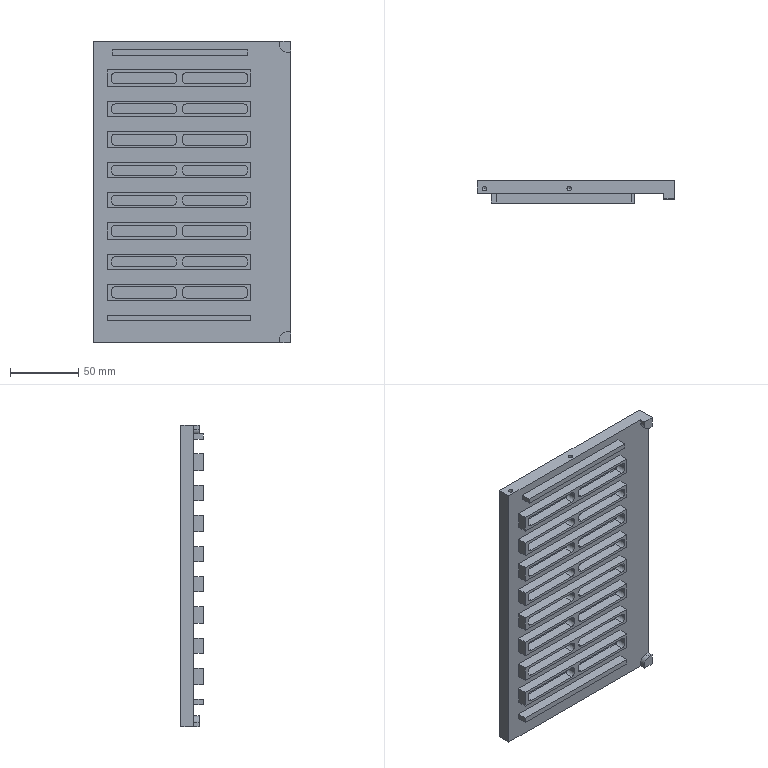NC program | NX | posted with a generic post | part box 144.5 x 16.5 x 221 mm
Lines 28 to 872 of 2050:
(PLANAR_MILL_9_COPY , TOOL : D2-6-D4-50-3T-FINISH)
N48 T13 M6
N50 G54
N52 G17 G0 G90 X66.787 Y-5.37 S4500 M3
N54 G43 Z20. H13
N56 Z1.
N58 G94 G1 X66.766 Y-5.373 Z0.998 F600.
N60 X66.624 Y-5.434 Z0.985
N62 X66.499 Y-5.527 Z0.971
N64 X66.401 Y-5.647 Z0.957
N66 X66.333 Y-5.786 Z0.944
N68 X66.3 Y-5.937 Z0.93
N70 Y-6.063 Z0.919
N72 X66.333 Y-6.214 Z0.906
N74 X66.401 Y-6.353 Z0.892
N76 X66.499 Y-6.473 Z0.879
N78 X66.624 Y-6.566 Z0.865
N80 X66.766 Y-6.627 Z0.852
N82 X66.919 Y-6.652 Z0.838
N84 X67.073 Y-6.641 Z0.825
N86 X67.221 Y-6.594 Z0.811
N88 X67.329 Y-6.532 Z0.8
N90 X67.433 Y-6.439 Z0.788
N92 X67.516 Y-6.327 Z0.776
N94 X67.572 Y-6.199 Z0.763
N96 X67.6 Y-6.063 Z0.751
N98 Y-5.937 Z0.74
N100 X67.572 Y-5.801 Z0.728
N102 X67.516 Y-5.674 Z0.716
N104 X67.433 Y-5.561 Z0.704
N106 X67.329 Y-5.468 Z0.692
N108 X67.221 Y-5.406 Z0.681
N110 X67.073 Y-5.359 Z0.667
N112 X66.919 Y-5.348 Z0.654
N114 X66.766 Y-5.373 Z0.64
N116 X66.624 Y-5.434 Z0.626
N118 X66.499 Y-5.527 Z0.613
N120 X66.401 Y-5.647 Z0.599
N122 X66.333 Y-5.786 Z0.586
N124 X66.3 Y-5.937 Z0.572
N126 Y-6.063 Z0.561
N128 X66.333 Y-6.214 Z0.548
N130 X66.401 Y-6.353 Z0.534
N132 X66.499 Y-6.473 Z0.521
N134 X66.624 Y-6.566 Z0.507
N136 X66.766 Y-6.627 Z0.493
N138 X66.919 Y-6.652 Z0.48
N140 X67.073 Y-6.641 Z0.466
N142 X67.221 Y-6.594 Z0.453
N144 X67.329 Y-6.532 Z0.442
N146 X67.433 Y-6.439 Z0.43
N148 X67.516 Y-6.327 Z0.417
N150 X67.572 Y-6.199 Z0.405
N152 X67.6 Y-6.063 Z0.393
N154 Y-5.937 Z0.382
N156 X67.572 Y-5.801 Z0.37
N158 X67.516 Y-5.674 Z0.358
N160 X67.433 Y-5.561 Z0.346
N162 X67.329 Y-5.468 Z0.333
N164 X67.221 Y-5.406 Z0.322
N166 X67.073 Y-5.359 Z0.309
N168 X66.919 Y-5.348 Z0.295
N170 X66.766 Y-5.373 Z0.282
N172 X66.624 Y-5.434 Z0.268
N174 X66.499 Y-5.527 Z0.255
N176 X66.401 Y-5.647 Z0.241
N178 X66.333 Y-5.786 Z0.228
N180 X66.3 Y-5.937 Z0.214
N182 Y-6.063 Z0.203
N184 X66.333 Y-6.214 Z0.189
N186 X66.401 Y-6.353 Z0.176
N188 X66.499 Y-6.473 Z0.162
N190 X66.624 Y-6.566 Z0.149
N192 X66.766 Y-6.627 Z0.135
N194 X66.919 Y-6.652 Z0.122
N196 X67.073 Y-6.641 Z0.108
N198 X67.221 Y-6.594 Z0.095
N200 X67.329 Y-6.532 Z0.084
N202 X67.433 Y-6.439 Z0.071
N204 X67.516 Y-6.327 Z0.059
N206 X67.572 Y-6.199 Z0.047
N208 X67.6 Y-6.063 Z0.035
N210 Y-5.937 Z0.024
N212 X67.572 Y-5.801 Z0.012
N214 X67.516 Y-5.674 Z0.
N216 X67.433 Y-5.561 Z-0.013
N218 X67.329 Y-5.468 Z-0.025
N220 X67.221 Y-5.406 Z-0.036
N222 X67.073 Y-5.359 Z-0.049
N224 X66.919 Y-5.348 Z-0.063
N226 X66.766 Y-5.373 Z-0.076
N228 X66.624 Y-5.434 Z-0.09
N230 X66.499 Y-5.527 Z-0.104
N232 X66.401 Y-5.647 Z-0.117
N234 X66.333 Y-5.786 Z-0.131
N236 X66.3 Y-5.937 Z-0.144
N238 Y-6.063 Z-0.155
N240 X66.333 Y-6.214 Z-0.169
N242 X66.401 Y-6.353 Z-0.182
N244 X66.499 Y-6.473 Z-0.196
N246 X66.624 Y-6.566 Z-0.209
N248 X66.766 Y-6.627 Z-0.223
N250 X66.919 Y-6.652 Z-0.236
N252 X67.073 Y-6.641 Z-0.25
N254 X67.221 Y-6.594 Z-0.264
N256 X67.329 Y-6.532 Z-0.275
N258 X67.433 Y-6.439 Z-0.287
N260 X67.516 Y-6.327 Z-0.299
N262 X67.572 Y-6.199 Z-0.311
N264 X67.6 Y-6.063 Z-0.323
N266 Y-5.937 Z-0.334
N268 X67.572 Y-5.801 Z-0.346
N270 X67.516 Y-5.674 Z-0.359
N272 X67.433 Y-5.561 Z-0.371
N274 X67.329 Y-5.468 Z-0.383
N276 X67.221 Y-5.406 Z-0.394
N278 X67.073 Y-5.359 Z-0.408
N280 X66.919 Y-5.348 Z-0.421
N282 X66.766 Y-5.373 Z-0.435
N284 X66.624 Y-5.434 Z-0.448
N286 X66.499 Y-5.527 Z-0.462
N288 X66.401 Y-5.647 Z-0.475
N290 X66.333 Y-5.786 Z-0.489
N292 X66.3 Y-5.937 Z-0.502
N294 Y-6.063 Z-0.513
N296 X66.333 Y-6.214 Z-0.527
N298 X66.401 Y-6.353 Z-0.54
N300 X66.499 Y-6.473 Z-0.554
N302 X66.624 Y-6.566 Z-0.568
N304 X66.766 Y-6.627 Z-0.581
N306 X66.919 Y-6.652 Z-0.595
N308 X67.073 Y-6.641 Z-0.608
N310 X67.221 Y-6.594 Z-0.622
N312 X67.329 Y-6.532 Z-0.633
N314 X67.433 Y-6.439 Z-0.645
N316 X67.516 Y-6.327 Z-0.657
N318 X67.572 Y-6.199 Z-0.669
N320 X67.6 Y-6.063 Z-0.681
N322 Y-5.937 Z-0.692
N324 X67.572 Y-5.801 Z-0.705
N326 X67.516 Y-5.674 Z-0.717
N328 X67.433 Y-5.561 Z-0.729
N330 X67.329 Y-5.468 Z-0.741
N332 X67.221 Y-5.406 Z-0.752
N334 X67.073 Y-5.359 Z-0.766
N336 X66.919 Y-5.348 Z-0.779
N338 X66.766 Y-5.373 Z-0.793
N340 X66.624 Y-5.434 Z-0.806
N342 X66.499 Y-5.527 Z-0.82
N344 X66.401 Y-5.647 Z-0.833
N346 X66.333 Y-5.786 Z-0.847
N348 X66.3 Y-5.937 Z-0.861
N350 Y-6.063 Z-0.872
N352 X66.333 Y-6.214 Z-0.885
N354 X66.401 Y-6.353 Z-0.899
N356 X66.499 Y-6.473 Z-0.912
N358 X66.624 Y-6.566 Z-0.926
N360 X66.766 Y-6.627 Z-0.939
N362 X66.919 Y-6.652 Z-0.953
N364 X67.073 Y-6.641 Z-0.966
N366 X67.221 Y-6.594 Z-0.98
N368 X67.329 Y-6.532 Z-0.991
N370 X67.433 Y-6.439 Z-1.003
N372 X67.516 Y-6.327 Z-1.015
N374 X67.572 Y-6.199 Z-1.027
N376 X67.6 Y-6.063 Z-1.04
N378 Y-5.937 Z-1.051
N380 X67.572 Y-5.801 Z-1.063
N382 X67.516 Y-5.674 Z-1.075
N384 X67.433 Y-5.561 Z-1.087
N386 X67.329 Y-5.468 Z-1.099
N388 X67.221 Y-5.406 Z-1.11
N390 X67.073 Y-5.359 Z-1.124
N392 X66.919 Y-5.348 Z-1.137
N394 X66.766 Y-5.373 Z-1.151
N396 X66.624 Y-5.434 Z-1.165
N398 X66.499 Y-5.527 Z-1.178
N400 X66.401 Y-5.647 Z-1.192
N402 X66.333 Y-5.786 Z-1.205
N404 X66.3 Y-5.937 Z-1.219
N406 Y-6.063 Z-1.23
N408 X66.333 Y-6.214 Z-1.243
N410 X66.401 Y-6.353 Z-1.257
N412 X66.499 Y-6.473 Z-1.27
N414 X66.624 Y-6.566 Z-1.284
N416 X66.766 Y-6.627 Z-1.297
N418 X66.919 Y-6.652 Z-1.311
N420 X67.073 Y-6.641 Z-1.325
N422 X67.221 Y-6.594 Z-1.338
N424 X67.329 Y-6.532 Z-1.349
N426 X67.433 Y-6.439 Z-1.361
N428 X67.516 Y-6.327 Z-1.373
N430 X67.572 Y-6.199 Z-1.386
N432 X67.6 Y-6.063 Z-1.398
N434 Y-5.937 Z-1.409
N436 X67.572 Y-5.801 Z-1.421
N438 X67.516 Y-5.674 Z-1.433
N440 X67.433 Y-5.561 Z-1.445
N442 X67.329 Y-5.468 Z-1.458
N444 X67.221 Y-5.406 Z-1.469
N446 X67.073 Y-5.359 Z-1.482
N448 X66.919 Y-5.348 Z-1.496
N450 X66.766 Y-5.373 Z-1.509
N452 X66.624 Y-5.434 Z-1.523
N454 X66.499 Y-5.527 Z-1.536
N456 X66.401 Y-5.647 Z-1.55
N458 X66.333 Y-5.786 Z-1.563
N460 X66.3 Y-5.937 Z-1.577
N462 Y-6.063 Z-1.588
N464 X66.333 Y-6.214 Z-1.601
N466 X66.401 Y-6.353 Z-1.615
N468 X66.499 Y-6.473 Z-1.629
N470 X66.624 Y-6.566 Z-1.642
N472 X66.766 Y-6.627 Z-1.656
N474 X66.919 Y-6.652 Z-1.669
N476 X67.073 Y-6.641 Z-1.683
N478 X67.221 Y-6.594 Z-1.696
N480 X67.329 Y-6.532 Z-1.707
N482 X67.433 Y-6.439 Z-1.719
N484 X67.516 Y-6.327 Z-1.732
N486 X67.572 Y-6.199 Z-1.744
N488 X67.6 Y-6.063 Z-1.756
N490 Y-5.937 Z-1.767
N492 X67.572 Y-5.801 Z-1.779
N494 X67.516 Y-5.674 Z-1.791
N496 X67.433 Y-5.561 Z-1.804
N498 X67.329 Y-5.468 Z-1.816
N500 X67.221 Y-5.406 Z-1.827
N502 X67.073 Y-5.359 Z-1.84
N504 X66.919 Y-5.348 Z-1.854
N506 X66.766 Y-5.373 Z-1.867
N508 X66.624 Y-5.434 Z-1.881
N510 X66.499 Y-5.527 Z-1.895
N512 X66.401 Y-5.647 Z-1.908
N514 X66.333 Y-5.786 Z-1.922
N516 X66.3 Y-5.937 Z-1.935
N518 Y-6.063 Z-1.946
N520 X66.333 Y-6.214 Z-1.96
N522 X66.401 Y-6.353 Z-1.973
N524 X66.499 Y-6.473 Z-1.987
N526 X66.624 Y-6.566 Z-2.
N528 X66.766 Y-6.627 Z-2.014
N530 X66.919 Y-6.652 Z-2.027
N532 X67.073 Y-6.641 Z-2.041
N534 X67.221 Y-6.594 Z-2.055
N536 X67.329 Y-6.532 Z-2.065
N538 X67.433 Y-6.439 Z-2.078
N540 X67.516 Y-6.327 Z-2.09
N542 X67.572 Y-6.199 Z-2.102
N544 X67.6 Y-6.063 Z-2.114
N546 Y-5.937 Z-2.125
N548 X67.572 Y-5.801 Z-2.137
N550 X67.516 Y-5.674 Z-2.15
N552 X67.433 Y-5.561 Z-2.162
N554 X67.329 Y-5.468 Z-2.174
N556 X67.221 Y-5.406 Z-2.185
N558 X67.073 Y-5.359 Z-2.198
N560 X66.919 Y-5.348 Z-2.212
N562 X66.766 Y-5.373 Z-2.226
N564 X66.624 Y-5.434 Z-2.239
N566 X66.499 Y-5.527 Z-2.253
N568 X66.401 Y-5.647 Z-2.266
N570 X66.333 Y-5.786 Z-2.28
N572 X66.3 Y-5.937 Z-2.293
N574 Y-6.063 Z-2.304
N576 X66.333 Y-6.214 Z-2.318
N578 X66.401 Y-6.353 Z-2.331
N580 X66.499 Y-6.473 Z-2.345
N582 X66.624 Y-6.566 Z-2.359
N584 X66.766 Y-6.627 Z-2.372
N586 X66.919 Y-6.652 Z-2.386
N588 X67.073 Y-6.641 Z-2.399
N590 X67.221 Y-6.594 Z-2.413
N592 X67.329 Y-6.532 Z-2.424
N594 X67.433 Y-6.439 Z-2.436
N596 X67.516 Y-6.327 Z-2.448
N598 X67.572 Y-6.199 Z-2.46
N600 X67.6 Y-6.063 Z-2.472
N602 Y-5.937 Z-2.483
N604 X67.572 Y-5.801 Z-2.496
N606 X67.516 Y-5.674 Z-2.508
N608 X67.433 Y-5.561 Z-2.52
N610 X67.329 Y-5.468 Z-2.532
N612 X67.221 Y-5.406 Z-2.543
N614 X67.073 Y-5.359 Z-2.557
N616 X66.919 Y-5.348 Z-2.57
N618 X66.766 Y-5.373 Z-2.584
N620 X66.624 Y-5.434 Z-2.597
N622 X66.499 Y-5.527 Z-2.611
N624 X66.401 Y-5.647 Z-2.624
N626 X66.333 Y-5.786 Z-2.638
N628 X66.3 Y-5.937 Z-2.652
N630 Y-6.063 Z-2.662
N632 X66.333 Y-6.214 Z-2.676
N634 X66.401 Y-6.353 Z-2.69
N636 X66.499 Y-6.473 Z-2.703
N638 X66.624 Y-6.566 Z-2.717
N640 X66.766 Y-6.627 Z-2.73
N642 X66.919 Y-6.652 Z-2.744
N644 X67.073 Y-6.641 Z-2.757
N646 X67.221 Y-6.594 Z-2.771
N648 X67.329 Y-6.532 Z-2.782
N650 X67.433 Y-6.439 Z-2.794
N652 X67.516 Y-6.327 Z-2.806
N654 X67.572 Y-6.199 Z-2.818
N656 X67.6 Y-6.063 Z-2.831
N658 Y-5.937 Z-2.842
N660 X67.572 Y-5.801 Z-2.854
N662 X67.516 Y-5.674 Z-2.866
N664 X67.433 Y-5.561 Z-2.878
N666 X67.329 Y-5.468 Z-2.89
N668 X67.221 Y-5.406 Z-2.901
N670 X67.073 Y-5.359 Z-2.915
N672 X66.919 Y-5.348 Z-2.928
N674 X66.766 Y-5.373 Z-2.942
N676 X66.624 Y-5.434 Z-2.956
N678 X66.499 Y-5.527 Z-2.969
N680 X66.401 Y-5.647 Z-2.983
N682 X66.333 Y-5.786 Z-2.996
N684 X66.3 Y-5.937 Z-3.01
N686 Y-6.063 Z-3.021
N688 X66.333 Y-6.214 Z-3.034
N690 X66.401 Y-6.353 Z-3.048
N692 X66.499 Y-6.473 Z-3.061
N694 X66.624 Y-6.566 Z-3.075
N696 X66.766 Y-6.627 Z-3.088
N698 X66.919 Y-6.652 Z-3.102
N700 X67.073 Y-6.641 Z-3.116
N702 X67.221 Y-6.594 Z-3.129
N704 X67.329 Y-6.532 Z-3.14
N706 X67.433 Y-6.439 Z-3.152
N708 X67.516 Y-6.327 Z-3.164
N710 X67.572 Y-6.199 Z-3.177
N712 X67.6 Y-6.063 Z-3.189
N714 Y-5.937 Z-3.2
N716 X67.572 Y-5.801 Z-3.212
N718 X67.516 Y-5.674 Z-3.224
N720 X67.433 Y-5.561 Z-3.236
N722 X67.329 Y-5.468 Z-3.249
N724 X67.221 Y-5.406 Z-3.26
N726 X67.073 Y-5.359 Z-3.273
N728 X66.919 Y-5.348 Z-3.287
N730 X66.766 Y-5.373 Z-3.3
N732 X66.624 Y-5.434 Z-3.314
N734 X66.499 Y-5.527 Z-3.327
N736 X66.401 Y-5.647 Z-3.341
N738 X66.333 Y-5.786 Z-3.354
N740 X66.3 Y-5.937 Z-3.368
N742 Y-6.063 Z-3.379
N744 X66.333 Y-6.214 Z-3.392
N746 X66.401 Y-6.353 Z-3.406
N748 X66.499 Y-6.473 Z-3.42
N750 X66.624 Y-6.566 Z-3.433
N752 X66.766 Y-6.627 Z-3.447
N754 X66.919 Y-6.652 Z-3.46
N756 X67.073 Y-6.641 Z-3.474
N758 X67.221 Y-6.594 Z-3.487
N760 X67.329 Y-6.532 Z-3.498
N762 X67.433 Y-6.439 Z-3.51
N764 X67.516 Y-6.327 Z-3.523
N766 X67.572 Y-6.199 Z-3.535
N768 X67.6 Y-6.063 Z-3.547
N770 Y-5.937 Z-3.558
N772 X67.572 Y-5.801 Z-3.57
N774 X67.516 Y-5.674 Z-3.582
N776 X67.433 Y-5.561 Z-3.595
N778 X67.329 Y-5.468 Z-3.607
N780 X67.221 Y-5.406 Z-3.618
N782 X67.073 Y-5.359 Z-3.631
N784 X66.919 Y-5.348 Z-3.645
N786 X66.766 Y-5.373 Z-3.658
N788 X66.624 Y-5.434 Z-3.672
N790 X66.499 Y-5.527 Z-3.685
N792 X66.401 Y-5.647 Z-3.699
N794 X66.333 Y-5.786 Z-3.713
N796 X66.3 Y-5.937 Z-3.726
N798 Y-6.063 Z-3.737
N800 X66.333 Y-6.214 Z-3.751
N802 X66.401 Y-6.353 Z-3.764
N804 X66.499 Y-6.473 Z-3.778
N806 X66.624 Y-6.566 Z-3.791
N808 X66.766 Y-6.627 Z-3.805
N810 X66.919 Y-6.652 Z-3.818
N812 X67.073 Y-6.641 Z-3.832
N814 X67.221 Y-6.594 Z-3.846
N816 X67.329 Y-6.532 Z-3.856
N818 X67.433 Y-6.439 Z-3.869
N820 X67.516 Y-6.327 Z-3.881
N822 X67.572 Y-6.199 Z-3.893
N824 X67.6 Y-6.063 Z-3.905
N826 Y-5.937 Z-3.916
N828 X67.572 Y-5.801 Z-3.928
N830 X67.516 Y-5.674 Z-3.941
N832 X67.433 Y-5.561 Z-3.953
N834 X67.329 Y-5.468 Z-3.965
N836 X67.221 Y-5.406 Z-3.976
N838 X67.073 Y-5.359 Z-3.989
N840 X66.919 Y-5.348 Z-4.003
N842 X66.766 Y-5.373 Z-4.017
N844 X66.624 Y-5.434 Z-4.03
N846 X66.499 Y-5.527 Z-4.044
N848 X66.401 Y-5.647 Z-4.057
N850 X66.333 Y-5.786 Z-4.071
N852 X66.3 Y-5.937 Z-4.084
N854 Y-6.063 Z-4.095
N856 X66.333 Y-6.214 Z-4.109
N858 X66.401 Y-6.353 Z-4.122
N860 X66.499 Y-6.473 Z-4.136
N862 X66.624 Y-6.566 Z-4.149
N864 X66.766 Y-6.627 Z-4.163
N866 X66.919 Y-6.652 Z-4.177
N868 X67.073 Y-6.641 Z-4.19
N870 X67.221 Y-6.594 Z-4.204
N872 X67.329 Y-6.532 Z-4.215
N874 X67.433 Y-6.439 Z-4.227
N876 X67.516 Y-6.327 Z-4.239
N878 X67.572 Y-6.199 Z-4.251
N880 X67.6 Y-6.063 Z-4.263
N882 Y-5.937 Z-4.274
N884 X67.572 Y-5.801 Z-4.287
N886 X67.516 Y-5.674 Z-4.299
N888 X67.433 Y-5.561 Z-4.311
N890 X67.329 Y-5.468 Z-4.323
N892 X67.221 Y-5.406 Z-4.334
N894 X67.073 Y-5.359 Z-4.348
N896 X66.919 Y-5.348 Z-4.361
N898 X66.766 Y-5.373 Z-4.375
N900 X66.624 Y-5.434 Z-4.388
N902 X66.499 Y-5.527 Z-4.402
N904 X66.401 Y-5.647 Z-4.415
N906 X66.333 Y-5.786 Z-4.429
N908 X66.3 Y-5.937 Z-4.443
N910 Y-6.063 Z-4.453
N912 X66.333 Y-6.214 Z-4.467
N914 X66.401 Y-6.353 Z-4.481
N916 X66.499 Y-6.473 Z-4.494
N918 X66.624 Y-6.566 Z-4.508
N920 X66.766 Y-6.627 Z-4.521
N922 X66.919 Y-6.652 Z-4.535
N924 X67.073 Y-6.641 Z-4.548
N926 X67.221 Y-6.594 Z-4.562
N928 X67.329 Y-6.532 Z-4.573
N930 X67.433 Y-6.439 Z-4.585
N932 X67.516 Y-6.327 Z-4.597
N934 X67.572 Y-6.199 Z-4.609
N936 X67.6 Y-6.063 Z-4.622
N938 Y-5.937 Z-4.633
N940 X67.572 Y-5.801 Z-4.645
N942 X67.516 Y-5.674 Z-4.657
N944 X67.433 Y-5.561 Z-4.669
N946 X67.329 Y-5.468 Z-4.681
N948 X67.221 Y-5.406 Z-4.692
N950 X67.073 Y-5.359 Z-4.706
N952 X66.919 Y-5.348 Z-4.719
N954 X66.766 Y-5.373 Z-4.733
N956 X66.624 Y-5.434 Z-4.747
N958 X66.499 Y-5.527 Z-4.76
N960 X66.401 Y-5.647 Z-4.774
N962 X66.333 Y-5.786 Z-4.787
N964 X66.3 Y-5.937 Z-4.801
N966 Y-6.063 Z-4.812
N968 X66.333 Y-6.214 Z-4.825
N970 X66.401 Y-6.353 Z-4.839
N972 X66.499 Y-6.473 Z-4.852
N974 X66.624 Y-6.566 Z-4.866
N976 X66.766 Y-6.627 Z-4.879
N978 X66.919 Y-6.652 Z-4.893
N980 X67.073 Y-6.641 Z-4.907
N982 X67.221 Y-6.594 Z-4.92
N984 X67.329 Y-6.532 Z-4.931
N986 X67.433 Y-6.439 Z-4.943
N988 X67.516 Y-6.327 Z-4.955
N990 X67.572 Y-6.199 Z-4.968
N992 X67.6 Y-6.063 Z-4.98
N994 Y-5.937 Z-4.991
N996 X67.572 Y-5.801 Z-5.003
N998 X67.516 Y-5.674 Z-5.015
N1000 X67.433 Y-5.561 Z-5.027
N1002 X67.329 Y-5.468 Z-5.04
N1004 X67.221 Y-5.406 Z-5.05
N1006 X67.073 Y-5.359 Z-5.064
N1008 X66.919 Y-5.348 Z-5.078
N1010 X66.766 Y-5.373 Z-5.091
N1012 X66.624 Y-5.434 Z-5.105
N1014 X66.499 Y-5.527 Z-5.118
N1016 X66.401 Y-5.647 Z-5.132
N1018 X66.333 Y-5.786 Z-5.145
N1020 X66.3 Y-5.937 Z-5.159
N1022 Y-6.063 Z-5.17
N1024 X66.333 Y-6.214 Z-5.183
N1026 X66.401 Y-6.353 Z-5.197
N1028 X66.499 Y-6.473 Z-5.211
N1030 X66.624 Y-6.566 Z-5.224
N1032 X66.766 Y-6.627 Z-5.238
N1034 X66.919 Y-6.652 Z-5.251
N1036 X67.073 Y-6.641 Z-5.265
N1038 X67.221 Y-6.594 Z-5.278
N1040 X67.329 Y-6.532 Z-5.289
N1042 X67.433 Y-6.439 Z-5.301
N1044 X67.516 Y-6.327 Z-5.314
N1046 X67.572 Y-6.199 Z-5.326
N1048 X67.6 Y-6.063 Z-5.338
N1050 Y-5.937 Z-5.349
N1052 X67.572 Y-5.801 Z-5.361
N1054 X67.516 Y-5.674 Z-5.373
N1056 X67.433 Y-5.561 Z-5.386
N1058 X67.329 Y-5.468 Z-5.398
N1060 X67.221 Y-5.406 Z-5.409
N1062 X67.073 Y-5.359 Z-5.422
N1064 X66.919 Y-5.348 Z-5.436
N1066 X66.766 Y-5.373 Z-5.449
N1068 X66.624 Y-5.434 Z-5.463
N1070 X66.499 Y-5.527 Z-5.476
N1072 X66.401 Y-5.647 Z-5.49
N1074 X66.333 Y-5.786 Z-5.504
N1076 X66.3 Y-5.937 Z-5.517
N1078 Y-6.063 Z-5.528
N1080 X66.333 Y-6.214 Z-5.542
N1082 X66.401 Y-6.353 Z-5.555
N1084 X66.499 Y-6.473 Z-5.569
N1086 X66.624 Y-6.566 Z-5.582
N1088 X66.766 Y-6.627 Z-5.596
N1090 X66.919 Y-6.652 Z-5.609
N1092 X67.073 Y-6.641 Z-5.623
N1094 X67.221 Y-6.594 Z-5.636
N1096 X67.329 Y-6.532 Z-5.647
N1098 X67.433 Y-6.439 Z-5.66
N1100 X67.516 Y-6.327 Z-5.672
N1102 X67.572 Y-6.199 Z-5.684
N1104 X67.6 Y-6.063 Z-5.696
N1106 Y-5.937 Z-5.707
N1108 X67.572 Y-5.801 Z-5.719
N1110 X67.516 Y-5.674 Z-5.732
N1112 X67.433 Y-5.561 Z-5.744
N1114 X67.329 Y-5.468 Z-5.756
N1116 X67.221 Y-5.406 Z-5.767
N1118 X67.073 Y-5.359 Z-5.78
N1120 X66.919 Y-5.348 Z-5.794
N1122 X66.766 Y-5.373 Z-5.808
N1124 X66.624 Y-5.434 Z-5.821
N1126 X66.499 Y-5.527 Z-5.835
N1128 X66.401 Y-5.647 Z-5.848
N1130 X66.333 Y-5.786 Z-5.862
N1132 X66.3 Y-5.937 Z-5.875
N1134 Y-6.063 Z-5.886
N1136 X66.333 Y-6.214 Z-5.9
N1138 X66.401 Y-6.353 Z-5.913
N1140 X66.499 Y-6.473 Z-5.927
N1142 X66.624 Y-6.566 Z-5.94
N1144 X66.766 Y-6.627 Z-5.954
N1146 X66.919 Y-6.652 Z-5.968
N1148 X67.073 Y-6.641 Z-5.981
N1150 X67.221 Y-6.594 Z-5.995
N1152 X67.329 Y-6.532 Z-6.006
N1154 X67.433 Y-6.439 Z-6.018
N1156 X67.516 Y-6.327 Z-6.03
N1158 X67.572 Y-6.199 Z-6.042
N1160 X67.6 Y-6.063 Z-6.054
N1162 Y-5.937 Z-6.065
N1164 X67.572 Y-5.801 Z-6.078
N1166 X67.516 Y-5.674 Z-6.09
N1168 X67.433 Y-5.561 Z-6.102
N1170 X67.329 Y-5.468 Z-6.114
N1172 X67.221 Y-5.406 Z-6.125
N1174 X67.073 Y-5.359 Z-6.139
N1176 X66.919 Y-5.348 Z-6.152
N1178 X66.766 Y-5.373 Z-6.166
N1180 X66.624 Y-5.434 Z-6.179
N1182 X66.499 Y-5.527 Z-6.193
N1184 X66.401 Y-5.647 Z-6.206
N1186 X66.333 Y-5.786 Z-6.22
N1188 X66.3 Y-5.937 Z-6.233
N1190 Y-6.063 Z-6.244
N1192 X66.333 Y-6.214 Z-6.258
N1194 X66.401 Y-6.353 Z-6.272
N1196 X66.499 Y-6.473 Z-6.285
N1198 X66.624 Y-6.566 Z-6.299
N1200 X66.766 Y-6.627 Z-6.312
N1202 X66.919 Y-6.652 Z-6.326
N1204 X67.073 Y-6.641 Z-6.339
N1206 X67.221 Y-6.594 Z-6.353
N1208 X67.329 Y-6.532 Z-6.364
N1210 X67.433 Y-6.439 Z-6.376
N1212 X67.516 Y-6.327 Z-6.388
N1214 X67.572 Y-6.199 Z-6.4
N1216 X67.6 Y-6.063 Z-6.413
N1218 Y-5.937 Z-6.424
N1220 X67.572 Y-5.801 Z-6.436
N1222 X67.516 Y-5.674 Z-6.448
N1224 X67.433 Y-5.561 Z-6.46
N1226 X67.329 Y-5.468 Z-6.472
N1228 X67.221 Y-5.406 Z-6.483
N1230 X67.073 Y-5.359 Z-6.497
N1232 X66.919 Y-5.348 Z-6.51
N1234 X66.766 Y-5.373 Z-6.524
N1236 X66.624 Y-5.434 Z-6.537
N1238 X66.499 Y-5.527 Z-6.551
N1240 X66.401 Y-5.647 Z-6.565
N1242 X66.333 Y-5.786 Z-6.578
N1244 X66.3 Y-5.937 Z-6.592
N1246 Y-6.063 Z-6.603
N1248 X66.333 Y-6.214 Z-6.616
N1250 X66.401 Y-6.353 Z-6.63
N1252 X66.499 Y-6.473 Z-6.643
N1254 X66.624 Y-6.566 Z-6.657
N1256 X66.766 Y-6.627 Z-6.67
N1258 X66.919 Y-6.652 Z-6.684
N1260 X67.073 Y-6.641 Z-6.698
N1262 X67.221 Y-6.594 Z-6.711
N1264 X67.329 Y-6.532 Z-6.722
N1266 X67.433 Y-6.439 Z-6.734
N1268 X67.516 Y-6.327 Z-6.746
N1270 X67.572 Y-6.199 Z-6.759
N1272 X67.6 Y-6.063 Z-6.771
N1274 Y-5.937 Z-6.782
N1276 X67.572 Y-5.801 Z-6.794
N1278 X67.516 Y-5.674 Z-6.806
N1280 X67.433 Y-5.561 Z-6.818
N1282 X67.329 Y-5.468 Z-6.831
N1284 X67.221 Y-5.406 Z-6.841
N1286 X67.073 Y-5.359 Z-6.855
N1288 X66.919 Y-5.348 Z-6.869
N1290 X66.766 Y-5.373 Z-6.882
N1292 X66.624 Y-5.434 Z-6.896
N1294 X66.499 Y-5.527 Z-6.909
N1296 X66.401 Y-5.647 Z-6.923
N1298 X66.333 Y-5.786 Z-6.936
N1300 X66.3 Y-5.937 Z-6.95
N1302 Y-6.063 Z-6.961
N1304 X66.333 Y-6.214 Z-6.974
N1306 X66.401 Y-6.353 Z-6.988
N1308 X66.499 Y-6.473 Z-7.001
N1310 X66.624 Y-6.566 Z-7.015
N1312 X66.766 Y-6.627 Z-7.029
N1314 X66.919 Y-6.652 Z-7.042
N1316 X67.073 Y-6.641 Z-7.056
N1318 X67.221 Y-6.594 Z-7.069
N1320 X67.329 Y-6.532 Z-7.08
N1322 X67.433 Y-6.439 Z-7.092
N1324 X67.516 Y-6.327 Z-7.105
N1326 X67.572 Y-6.199 Z-7.117
N1328 X67.6 Y-6.063 Z-7.129
N1330 Y-5.937 Z-7.14
N1332 X67.572 Y-5.801 Z-7.152
N1334 X67.516 Y-5.674 Z-7.164
N1336 X67.433 Y-5.561 Z-7.177
N1338 X67.329 Y-5.468 Z-7.189
N1340 X67.221 Y-5.406 Z-7.2
N1342 X67.073 Y-5.359 Z-7.213
N1344 X66.919 Y-5.348 Z-7.227
N1346 X66.766 Y-5.373 Z-7.24
N1348 X66.624 Y-5.434 Z-7.254
N1350 X66.499 Y-5.527 Z-7.267
N1352 X66.401 Y-5.647 Z-7.281
N1354 X66.333 Y-5.786 Z-7.295
N1356 X66.3 Y-5.937 Z-7.308
N1358 Y-6.063 Z-7.319
N1360 X66.333 Y-6.214 Z-7.333
N1362 X66.401 Y-6.353 Z-7.346
N1364 X66.499 Y-6.473 Z-7.36
N1366 X66.624 Y-6.566 Z-7.373
N1368 X66.766 Y-6.627 Z-7.387
N1370 X66.919 Y-6.652 Z-7.4
N1372 X67.073 Y-6.641 Z-7.414
N1374 X67.221 Y-6.594 Z-7.427
N1376 X67.329 Y-6.532 Z-7.438
N1378 X67.433 Y-6.439 Z-7.451
N1380 X67.516 Y-6.327 Z-7.463
N1382 X67.572 Y-6.199 Z-7.475
N1384 X67.6 Y-6.063 Z-7.487
N1386 Y-5.937 Z-7.498
N1388 X67.572 Y-5.801 Z-7.51
N1390 X67.516 Y-5.674 Z-7.523
N1392 X67.433 Y-5.561 Z-7.535
N1394 X67.329 Y-5.468 Z-7.547
N1396 X67.221 Y-5.406 Z-7.558
N1398 X67.073 Y-5.359 Z-7.571
N1400 X66.919 Y-5.348 Z-7.585
N1402 X66.766 Y-5.373 Z-7.598
N1404 X66.624 Y-5.434 Z-7.612
N1406 X66.499 Y-5.527 Z-7.626
N1408 X66.401 Y-5.647 Z-7.639
N1410 X66.333 Y-5.786 Z-7.653
N1412 X66.3 Y-5.937 Z-7.666
N1414 Y-6.063 Z-7.677
N1416 X66.333 Y-6.214 Z-7.691
N1418 X66.401 Y-6.353 Z-7.704
N1420 X66.499 Y-6.473 Z-7.718
N1422 X66.624 Y-6.566 Z-7.731
N1424 X66.766 Y-6.627 Z-7.745
N1426 X66.919 Y-6.652 Z-7.759
N1428 X67.073 Y-6.641 Z-7.772
N1430 X67.221 Y-6.594 Z-7.786
N1432 X67.329 Y-6.532 Z-7.797
N1434 X67.433 Y-6.439 Z-7.809
N1436 X67.516 Y-6.327 Z-7.821
N1438 X67.572 Y-6.199 Z-7.833
N1440 X67.6 Y-6.063 Z-7.845
N1442 Y-5.937 Z-7.856
N1444 X67.572 Y-5.801 Z-7.869
N1446 X67.516 Y-5.674 Z-7.881
N1448 X67.433 Y-5.561 Z-7.893
N1450 X67.329 Y-5.468 Z-7.905
N1452 X67.221 Y-5.406 Z-7.916
N1454 X67.073 Y-5.359 Z-7.93
N1456 X66.919 Y-5.348 Z-7.943
N1458 X66.766 Y-5.373 Z-7.957
N1460 X66.624 Y-5.434 Z-7.97
N1462 X66.499 Y-5.527 Z-7.984
N1464 X66.401 Y-5.647 Z-7.997
N1466 X66.333 Y-5.786 Z-8.011
N1468 X66.3 Y-5.937 Z-8.024
N1470 Y-6.063 Z-8.035
N1472 X66.333 Y-6.214 Z-8.049
N1474 X66.401 Y-6.353 Z-8.063
N1476 X66.499 Y-6.473 Z-8.076
N1478 X66.624 Y-6.566 Z-8.09
N1480 X66.766 Y-6.627 Z-8.103
N1482 X66.919 Y-6.652 Z-8.117
N1484 X67.073 Y-6.641 Z-8.13
N1486 X67.221 Y-6.594 Z-8.144
N1488 X67.329 Y-6.532 Z-8.155
N1490 X67.433 Y-6.439 Z-8.167
N1492 X67.516 Y-6.327 Z-8.179
N1494 X67.572 Y-6.199 Z-8.191
N1496 X67.6 Y-6.063 Z-8.204
N1498 Y-5.937 Z-8.215
N1500 X67.572 Y-5.801 Z-8.227
N1502 X67.516 Y-5.674 Z-8.239
N1504 X67.433 Y-5.561 Z-8.251
N1506 X67.329 Y-5.468 Z-8.263
N1508 X67.221 Y-5.406 Z-8.274
N1510 X67.073 Y-5.359 Z-8.288
N1512 X66.919 Y-5.348 Z-8.301
N1514 X66.766 Y-5.373 Z-8.315
N1516 X66.624 Y-5.434 Z-8.328
N1518 X66.499 Y-5.527 Z-8.342
N1520 X66.401 Y-5.647 Z-8.356
N1522 X66.333 Y-5.786 Z-8.369
N1524 X66.3 Y-5.937 Z-8.383
N1526 Y-6.063 Z-8.394
N1528 X66.333 Y-6.214 Z-8.407
N1530 X66.401 Y-6.353 Z-8.421
N1532 X66.499 Y-6.473 Z-8.434
N1534 X66.624 Y-6.566 Z-8.448
N1536 X66.766 Y-6.627 Z-8.461
N1538 X66.919 Y-6.652 Z-8.475
N1540 X67.073 Y-6.641 Z-8.488
N1542 X67.221 Y-6.594 Z-8.502
N1544 X67.329 Y-6.532 Z-8.513
N1546 X67.433 Y-6.439 Z-8.525
N1548 X67.516 Y-6.327 Z-8.537
N1550 X67.572 Y-6.199 Z-8.55
N1552 X67.6 Y-6.063 Z-8.562
N1554 Y-5.937 Z-8.573
N1556 X67.572 Y-5.801 Z-8.585
N1558 X67.516 Y-5.674 Z-8.597
N1560 X67.433 Y-5.561 Z-8.609
N1562 X67.329 Y-5.468 Z-8.621
N1564 X67.221 Y-5.406 Z-8.632
N1566 X67.073 Y-5.359 Z-8.646
N1568 X66.919 Y-5.348 Z-8.66
N1570 X66.766 Y-5.373 Z-8.673
N1572 X66.624 Y-5.434 Z-8.687
N1574 X66.499 Y-5.527 Z-8.7
N1576 X66.401 Y-5.647 Z-8.714
N1578 X66.333 Y-5.786 Z-8.727
N1580 X66.3 Y-5.937 Z-8.741
N1582 Y-6.063 Z-8.752
N1584 X66.333 Y-6.214 Z-8.765
N1586 X66.401 Y-6.353 Z-8.779
N1588 X66.499 Y-6.473 Z-8.792
N1590 X66.624 Y-6.566 Z-8.806
N1592 X66.766 Y-6.627 Z-8.82
N1594 X66.919 Y-6.652 Z-8.833
N1596 X67.073 Y-6.641 Z-8.847
N1598 X67.221 Y-6.594 Z-8.86
N1600 X67.329 Y-6.532 Z-8.871
N1602 X67.433 Y-6.439 Z-8.883
N1604 X67.516 Y-6.327 Z-8.896
N1606 X67.572 Y-6.199 Z-8.908
N1608 X67.6 Y-6.063 Z-8.92
N1610 Y-5.937 Z-8.931
N1612 X67.572 Y-5.801 Z-8.943
N1614 X67.516 Y-5.674 Z-8.955
N1616 X67.433 Y-5.561 Z-8.967
N1618 X67.329 Y-5.468 Z-8.98
N1620 X67.221 Y-5.406 Z-8.991
N1622 X67.073 Y-5.359 Z-9.004
N1624 X66.919 Y-5.348 Z-9.018
N1626 X66.766 Y-5.373 Z-9.031
N1628 X66.624 Y-5.434 Z-9.045
N1630 X66.499 Y-5.527 Z-9.058
N1632 X66.401 Y-5.647 Z-9.072
N1634 X66.333 Y-5.786 Z-9.085
N1636 X66.3 Y-5.937 Z-9.099
N1638 Y-6.063 Z-9.11
N1640 X66.333 Y-6.214 Z-9.124
N1642 X66.401 Y-6.353 Z-9.137
N1644 X66.499 Y-6.473 Z-9.151
N1646 X66.624 Y-6.566 Z-9.164
N1648 X66.766 Y-6.627 Z-9.178
N1650 X66.919 Y-6.652 Z-9.191
N1652 X67.073 Y-6.641 Z-9.205
N1654 X67.221 Y-6.594 Z-9.218
N1656 X67.329 Y-6.532 Z-9.229
N1658 X67.433 Y-6.439 Z-9.242
N1660 X67.516 Y-6.327 Z-9.254
N1662 X67.572 Y-6.199 Z-9.266
N1664 X67.6 Y-6.063 Z-9.278
N1666 Y-5.937 Z-9.289
N1668 X67.572 Y-5.801 Z-9.301
N1670 X67.516 Y-5.674 Z-9.313
N1672 X67.433 Y-5.561 Z-9.326
N1674 X67.329 Y-5.468 Z-9.338
N1676 X67.221 Y-5.406 Z-9.349
N1678 X67.073 Y-5.359 Z-9.362
N1680 X66.919 Y-5.348 Z-9.376
N1682 X66.766 Y-5.373 Z-9.389
N1684 X66.624 Y-5.434 Z-9.403
N1686 X66.499 Y-5.527 Z-9.417
N1688 X66.401 Y-5.647 Z-9.43
N1690 X66.333 Y-5.786 Z-9.444
N1692 X66.3 Y-5.937 Z-9.457
N1694 Y-6.063 Z-9.468
N1696 X66.333 Y-6.214 Z-9.482
N1698 X66.401 Y-6.353 Z-9.495
N1700 X66.499 Y-6.473 Z-9.509
N1702 X66.624 Y-6.566 Z-9.522
N1704 X66.766 Y-6.627 Z-9.536
N1706 X66.919 Y-6.652 Z-9.55
N1708 X67.073 Y-6.641 Z-9.563
N1710 X67.221 Y-6.594 Z-9.577
N1712 X67.329 Y-6.532 Z-9.588
N1714 X67.433 Y-6.439 Z-9.6
N1716 X67.516 Y-6.327 Z-9.612
N1718 X67.572 Y-6.199 Z-9.624
N1720 X67.6 Y-6.063 Z-9.636
N1722 Y-5.937 Z-9.647
N1724 X67.572 Y-5.801 Z-9.659
N1726 X67.516 Y-5.674 Z-9.672
N1728 X67.433 Y-5.561 Z-9.684
N1730 X67.329 Y-5.468 Z-9.696